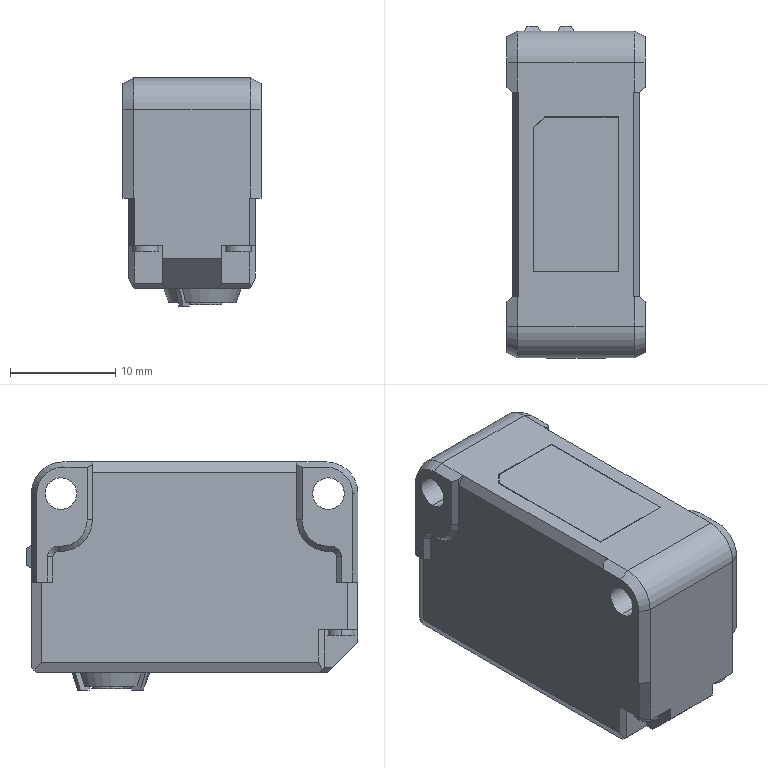Part | STEP file | PZ-G51EP-Part-5 | 1 solid | 210 faces | box 13.1 x 31.5 x 21.65 mm | volume 7176 mm3 | plane 120 | cylinder 74 | cone 16 | commonest cylinder face diameters 0.3 x25 0.5 x22 2.5 x6 6 x6 1 x4 3 x4